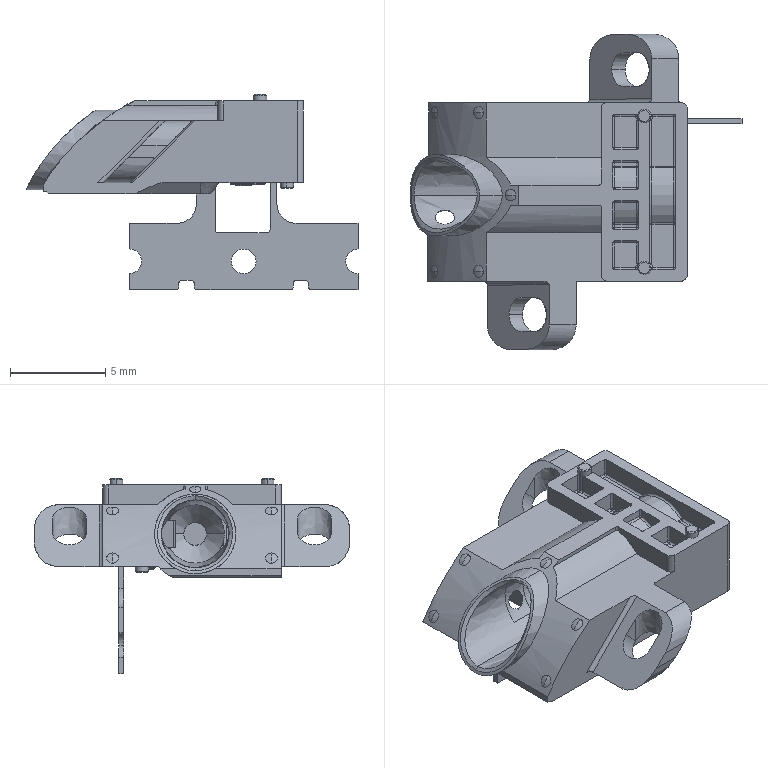Part | NX | 2 solids | 732 faces | box 17.419 x 16.558 x 10.278 mm | volume 297.015 mm3 | plane 367 | cylinder 237 | sphere 48 | torus 42 | spline 20 | cone 18 | commonest cylinder face diameters 0.2 x104 0.3 x16 0.4 x16 1 x15 0.7 x13 0.5 x6